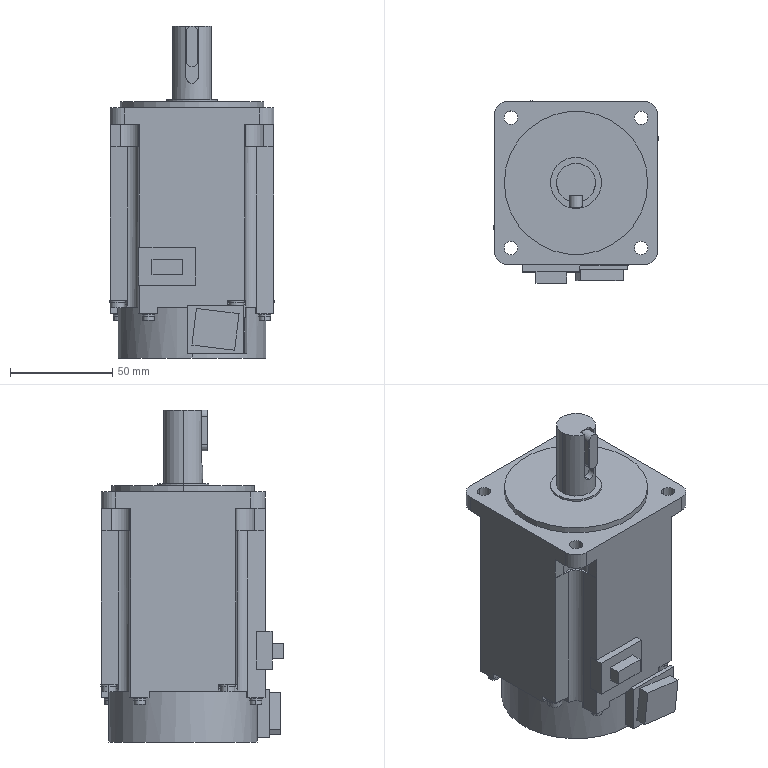Part | SolidWorks | features BaseBody 1, ICE 1, MoveCopyBody 1, Stock 1 | 2 solids | 215 faces | box 80.44 x 89.02 x 162.2 mm | volume 690586 mm3 | plane 117 | cylinder 98 | commonest cylinder face diameters 920 x17 6 x13 5.5 x8 5.9 x8 6.6 x8 7 x8